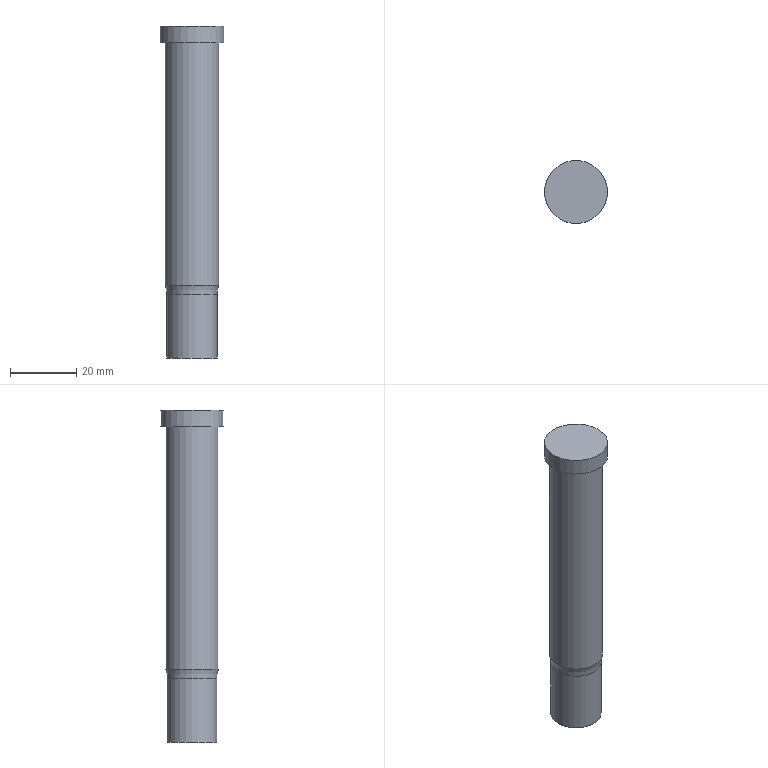Part | NX | features SPAS 16-80-15.10 2 | 1 solid | 7 faces | box 19 x 19 x 100 mm | volume 20057 mm3 | plane 3 | cylinder 3 | torus 1 | commonest cylinder face diameters 15.1 x1 16 x1 19 x1
STEP:
#1=CARTESIAN_POINT('',(332.81,-38.175,-22.));
#2=VERTEX_POINT('',#1);
#3=CARTESIAN_POINT('',(325.26,-38.175,-22.));
#4=DIRECTION('',(0.,0.,1.));
#5=DIRECTION('',(1.,0.,0.));
#6=AXIS2_PLACEMENT_3D('',#3,#4,#5);
#7=CIRCLE('',#6,7.55);
#8=EDGE_CURVE('',#2,#2,#7,.T.);
#9=ORIENTED_EDGE('',*,*,#8,.F.);
#10=EDGE_LOOP('',(#9));
#11=FACE_BOUND('',#10,.T.);
#12=CARTESIAN_POINT('',(325.26,-38.175,-22.));
#13=DIRECTION('',(0.,0.,-1.));
#14=DIRECTION('',(-1.,0.,0.));
#15=AXIS2_PLACEMENT_3D('',#12,#13,#14);
#16=PLANE('',#15);
#17=ADVANCED_FACE('',(#11),#16,.T.);
#18=CARTESIAN_POINT('',(332.81,-38.175,-3.));
#19=VERTEX_POINT('',#18);
#20=CARTESIAN_POINT('',(325.26,-38.175,-3.));
#21=DIRECTION('',(0.,0.,1.));
#22=DIRECTION('',(1.,0.,0.));
#23=AXIS2_PLACEMENT_3D('',#20,#21,#22);
#24=CIRCLE('',#23,7.55);
#25=EDGE_CURVE('',#19,#19,#24,.F.);
#26=ORIENTED_EDGE('',*,*,#25,.T.);
#27=EDGE_LOOP('',(#26));
#28=FACE_BOUND('',#27,.T.);
#29=ORIENTED_EDGE('',*,*,#8,.T.);
#30=EDGE_LOOP('',(#29));
#31=FACE_BOUND('',#30,.T.);
#32=CARTESIAN_POINT('',(325.26,-38.175,-22.));
#33=DIRECTION('',(0.,0.,1.));
#34=DIRECTION('',(1.,0.,0.));
#35=AXIS2_PLACEMENT_3D('',#32,#33,#34);
#36=CYLINDRICAL_SURFACE('',#35,7.55);
#37=ADVANCED_FACE('',(#28,#31),#36,.T.);
#38=CARTESIAN_POINT('',(317.26,-38.175,73.));
#39=VERTEX_POINT('',#38);
#40=CARTESIAN_POINT('',(325.26,-38.175,73.));
#41=DIRECTION('',(0.,0.,-1.));
#42=DIRECTION('',(-1.,0.,0.));
#43=AXIS2_PLACEMENT_3D('',#40,#41,#42);
#44=CIRCLE('',#43,8.);
#45=EDGE_CURVE('',#39,#39,#44,.F.);
#46=ORIENTED_EDGE('',*,*,#45,.F.);
#47=EDGE_LOOP('',(#46));
#48=FACE_BOUND('',#47,.T.);
#49=CARTESIAN_POINT('',(333.26,-38.175,-0.03394));
#50=VERTEX_POINT('',#49);
#51=CARTESIAN_POINT('',(325.26,-38.175,-0.03394));
#52=DIRECTION('',(0.,0.,1.));
#53=DIRECTION('',(1.,0.,0.));
#54=AXIS2_PLACEMENT_3D('',#51,#52,#53);
#55=CIRCLE('',#54,8.);
#56=EDGE_CURVE('',#50,#50,#55,.T.);
#57=ORIENTED_EDGE('',*,*,#56,.T.);
#58=EDGE_LOOP('',(#57));
#59=FACE_BOUND('',#58,.T.);
#60=CARTESIAN_POINT('',(325.26,-38.175,-0.03394));
#61=DIRECTION('',(0.,0.,1.));
#62=DIRECTION('',(1.,0.,0.));
#63=AXIS2_PLACEMENT_3D('',#60,#61,#62);
#64=CYLINDRICAL_SURFACE('',#63,8.);
#65=ADVANCED_FACE('',(#48,#59),#64,.T.);
#66=CARTESIAN_POINT('',(334.76,-38.175,78.));
#67=VERTEX_POINT('',#66);
#68=CARTESIAN_POINT('',(325.26,-38.175,78.));
#69=DIRECTION('',(0.,0.,1.));
#70=DIRECTION('',(1.,0.,0.));
#71=AXIS2_PLACEMENT_3D('',#68,#69,#70);
#72=CIRCLE('',#71,9.5);
#73=EDGE_CURVE('',#67,#67,#72,.F.);
#74=ORIENTED_EDGE('',*,*,#73,.F.);
#75=EDGE_LOOP('',(#74));
#76=FACE_BOUND('',#75,.T.);
#77=CARTESIAN_POINT('',(325.26,-38.175,78.));
#78=DIRECTION('',(0.,0.,1.));
#79=DIRECTION('',(1.,0.,0.));
#80=AXIS2_PLACEMENT_3D('',#77,#78,#79);
#81=PLANE('',#80);
#82=ADVANCED_FACE('',(#76),#81,.T.);
#83=ORIENTED_EDGE('',*,*,#45,.T.);
#84=EDGE_LOOP('',(#83));
#85=FACE_BOUND('',#84,.T.);
#86=CARTESIAN_POINT('',(315.76,-38.175,73.));
#87=VERTEX_POINT('',#86);
#88=CARTESIAN_POINT('',(325.26,-38.175,73.));
#89=DIRECTION('',(0.,0.,-1.));
#90=DIRECTION('',(-1.,0.,0.));
#91=AXIS2_PLACEMENT_3D('',#88,#89,#90);
#92=CIRCLE('',#91,9.5);
#93=EDGE_CURVE('',#87,#87,#92,.F.);
#94=ORIENTED_EDGE('',*,*,#93,.F.);
#95=EDGE_LOOP('',(#94));
#96=FACE_BOUND('',#95,.T.);
#97=CARTESIAN_POINT('',(325.26,-38.175,73.));
#98=DIRECTION('',(0.,0.,-1.));
#99=DIRECTION('',(-1.,0.,0.));
#100=AXIS2_PLACEMENT_3D('',#97,#98,#99);
#101=PLANE('',#100);
#102=ADVANCED_FACE('',(#85,#96),#101,.T.);
#103=ORIENTED_EDGE('',*,*,#73,.T.);
#104=EDGE_LOOP('',(#103));
#105=FACE_BOUND('',#104,.T.);
#106=ORIENTED_EDGE('',*,*,#93,.T.);
#107=EDGE_LOOP('',(#106));
#108=FACE_BOUND('',#107,.T.);
#109=CARTESIAN_POINT('',(325.26,-38.175,53.));
#110=DIRECTION('',(0.,0.,1.));
#111=DIRECTION('',(1.,0.,0.));
#112=AXIS2_PLACEMENT_3D('',#109,#110,#111);
#113=CYLINDRICAL_SURFACE('',#112,9.5);
#114=ADVANCED_FACE('',(#105,#108),#113,.T.);
#115=ORIENTED_EDGE('',*,*,#25,.F.);
#116=EDGE_LOOP('',(#115));
#117=FACE_BOUND('',#116,.T.);
#118=ORIENTED_EDGE('',*,*,#56,.F.);
#119=EDGE_LOOP('',(#118));
#120=FACE_BOUND('',#119,.T.);
#121=CARTESIAN_POINT('',(325.26,-38.175,-3.));
#122=DIRECTION('',(0.,0.,1.));
#123=DIRECTION('',(1.,0.,0.));
#124=AXIS2_PLACEMENT_3D('',#121,#122,#123);
#125=TOROIDAL_SURFACE('',#124,17.55,10.);
#126=ADVANCED_FACE('',(#117,#120),#125,.F.);
#127=CLOSED_SHELL('',(#17,#37,#65,#82,#102,#114,#126));
#128=MANIFOLD_SOLID_BREP('',#127);
#129=(LENGTH_UNIT()NAMED_UNIT(*)SI_UNIT(.MILLI.,.METRE.));
#130=UNCERTAINTY_MEASURE_WITH_UNIT(LENGTH_MEASURE(0.00001),#129,'','');
#131=(NAMED_UNIT(*)PLANE_ANGLE_UNIT()SI_UNIT($,.RADIAN.));
#132=(NAMED_UNIT(*)SI_UNIT($,.STERADIAN.)SOLID_ANGLE_UNIT());
#133=(GEOMETRIC_REPRESENTATION_CONTEXT(3)GLOBAL_UNCERTAINTY_ASSIGNED_CONTEXT((#130))GLOBAL_UNIT_ASSIGNED_CONTEXT((#129,#131,#132))REPRESENTATION_CONTEXT('',''));
#134=ADVANCED_BREP_SHAPE_REPRESENTATION('',(#128),#133);